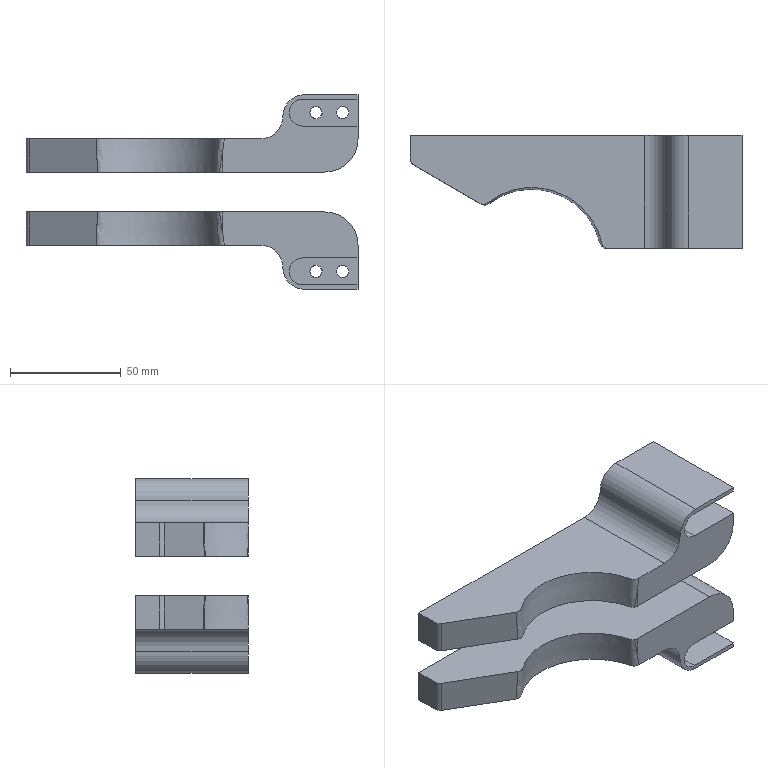NC program | NX | posted with a generic post | part box 150 x 51 x 88 mm
Lines 8834 to 9174 of 21241:
(ZLEVEL_PROFILE_COPY_COPY_COPY_1_COPY_COPY_COPY , TOOL : D12JING)
N17642 T11 M6
N17644 G54
N17646 G17 G0 G90 X62.688 Y-26.945 S9500 M3
N17648 G43 Z30. H11
N17650 Z-8.5
N17652 G94 G1 X61.043 Y-24.095 F1000.
N17654 G3 X60.005 Y-23.495 R1.199
N17656 G1 X-75. F1200.
N17658 G2 X-80.995 Y-17.5 R5.995
N17660 G1 Y-2.5
N17662 G2 X-75. Y3.495 R5.995
N17664 G1 X31.
N17666 G3 X35.005 Y7.5 R4.005
N17668 G2 X51. Y23.495 R15.995
N17670 G1 X75.
N17672 G2 X80.995 Y17.5 R5.995
N17674 G1 Y-2.5
N17676 G2 X60.005 Y-23.495 R20.995
N17678 G3 X58.966 Y-24.095 R1.199
N17680 G1 X57.237 Y-27.092
N17682 G0 X62.688 Y-26.945 Z-17.
N17684 G1 X61.043 Y-24.095 F1000.
N17686 G3 X60.005 Y-23.495 R1.199
N17688 G1 X-75. F1200.
N17690 G2 X-80.995 Y-17.5 R5.995
N17692 G1 Y-2.5
N17694 G2 X-75. Y3.495 R5.995
N17696 G1 X31.
N17698 G3 X35.005 Y7.5 R4.005
N17700 G2 X51. Y23.495 R15.995
N17702 G1 X75.
N17704 G2 X80.995 Y17.5 R5.995
N17706 G1 Y-2.5
N17708 G2 X60.005 Y-23.495 R20.995
N17710 G3 X58.966 Y-24.095 R1.199
N17712 G1 X57.237 Y-27.092
N17714 G0 X62.688 Y-26.945 Z-25.5
N17716 G1 X61.043 Y-24.095 F1000.
N17718 G3 X60.005 Y-23.495 R1.199
N17720 G1 X-75. F1200.
N17722 G2 X-80.995 Y-17.5 R5.995
N17724 G1 Y-2.5
N17726 G2 X-75. Y3.495 R5.995
N17728 G1 X31.
N17730 G3 X35.005 Y7.5 R4.005
N17732 G2 X51. Y23.495 R15.995
N17734 G1 X75.
N17736 G2 X80.995 Y17.5 R5.995
N17738 G1 Y-2.5
N17740 G2 X60.005 Y-23.495 R20.995
N17742 G3 X58.966 Y-24.095 R1.199
N17744 G1 X57.237 Y-27.092
N17746 G0 X62.688 Y-26.945 Z-34.
N17748 G1 X61.043 Y-24.095 F1000.
N17750 G3 X60.005 Y-23.495 R1.199
N17752 G1 X-75. F1200.
N17754 G2 X-80.995 Y-17.5 R5.995
N17756 G1 Y-2.5
N17758 G2 X-75. Y3.495 R5.995
N17760 G1 X31.
N17762 G3 X35.005 Y7.5 R4.005
N17764 G2 X51. Y23.495 R15.995
N17766 G1 X75.
N17768 G2 X80.995 Y17.5 R5.995
N17770 G1 Y-2.5
N17772 G2 X60.005 Y-23.495 R20.995
N17774 G3 X58.966 Y-24.095 R1.199
N17776 G1 X57.237 Y-27.092
N17778 G0 X62.688 Y-26.945 Z-42.5
N17780 G1 X61.043 Y-24.095 F1000.
N17782 G3 X60.005 Y-23.495 R1.199
N17784 G1 X-75. F1200.
N17786 G2 X-80.995 Y-17.5 R5.995
N17788 G1 Y-2.5
N17790 G2 X-75. Y3.495 R5.995
N17792 G1 X31.
N17794 G3 X35.005 Y7.5 R4.005
N17796 G2 X51. Y23.495 R15.995
N17798 G1 X75.
N17800 G2 X80.995 Y17.5 R5.995
N17802 G1 Y-2.5
N17804 G2 X60.005 Y-23.495 R20.995
N17806 G3 X58.966 Y-24.095 R1.199
N17808 G1 X57.237 Y-27.092
N17810 G0 X62.688 Y-26.945 Z-51.
N17812 G1 X61.043 Y-24.095 F1000.
N17814 G3 X60.005 Y-23.495 R1.199
N17816 G1 X-75. F1200.
N17818 G2 X-80.995 Y-17.5 R5.995
N17820 G1 Y-2.5
N17822 G2 X-75. Y3.495 R5.995
N17824 G1 X31.
N17826 G3 X35.005 Y7.5 R4.005
N17828 G2 X51. Y23.495 R15.995
N17830 G1 X75.
N17832 G2 X80.995 Y17.5 R5.995
N17834 G1 Y-2.5
N17836 G2 X60.005 Y-23.495 R20.995
N17838 G3 X58.966 Y-24.095 R1.199
N17840 G1 X57.237 Y-27.092
N17842 G0 Z30.
(ZLEVEL_PROFILE , TOOL : D12JING)
N17844 X81.455 Y9.508
N17846 Z0.
N17848 G1 Z-0.95 F1650.
N17850 X80.966 Y9.505
N17852 X74.609
N17854 X50.
N17856 G3 X49.895 Y9.4 R0.105
N17858 X50. Y9.295 R0.105
N17860 G1 X74.609
N17862 X80.966
N17864 X81.455 Y9.293
N17866 G3 X81.755 Y9.371 R0.6
N17868 G0 X81.455 Y9.508
N17870 G1 Z-1.9
N17872 X80.966 Y9.504
N17874 X74.609 Y9.505
N17876 X50.
N17878 G3 X49.895 Y9.4 R0.105
N17880 X50. Y9.295 R0.105
N17882 G1 X74.609
N17884 X80.966 Y9.296
N17886 X81.455 Y9.293
N17888 G3 X81.755 Y9.371 R0.6
N17890 G0 X81.455 Y9.508
N17892 G1 Z-2.85
N17894 X80.966 Y9.504
N17896 X74.609 Y9.505
N17898 X50.
N17900 G3 X49.895 Y9.4 R0.105
N17902 X50. Y9.295 R0.105
N17904 G1 X74.609
N17906 X80.966 Y9.296
N17908 X81.455 Y9.293
N17910 G3 X81.755 Y9.371 R0.6
N17912 G0 X81.455 Y9.508
N17914 G1 Z-3.8
N17916 X80.966 Y9.504
N17918 X75.098
N17920 X74.609 Y9.505
N17922 X50.
N17924 G3 X49.895 Y9.4 R0.105
N17926 X50. Y9.295 R0.105
N17928 G1 X74.609
N17930 X75.098 Y9.296
N17932 X80.966
N17934 X81.455 Y9.293
N17936 G3 X81.755 Y9.372 R0.6
N17938 G0 X81.455 Y9.508
N17940 G1 Z-4.75
N17942 X80.966 Y9.504
N17944 X75.098
N17946 X74.609 Y9.505
N17948 X50.
N17950 G3 X49.895 Y9.4 R0.105
N17952 X50. Y9.295 R0.105
N17954 G1 X74.609
N17956 X75.098 Y9.296
N17958 X80.966
N17960 X81.455 Y9.293
N17962 G3 X81.755 Y9.372 R0.6
N17964 G0 X81.455 Y9.508
N17966 G1 Z-5.7
N17968 X80.966 Y9.504
N17970 X75.098
N17972 X74.609 Y9.505
N17974 X50.
N17976 G3 X49.895 Y9.4 R0.105
N17978 X50. Y9.295 R0.105
N17980 G1 X74.609
N17982 X75.098 Y9.296
N17984 X80.966
N17986 X81.455 Y9.293
N17988 G3 X81.755 Y9.372 R0.6
N17990 G0 X81.455 Y9.507
N17992 G1 Z-6.65
N17994 X80.966 Y9.504
N17996 X75.098
N17998 X74.609 Y9.505
N18000 X50.
N18002 G3 X49.895 Y9.4 R0.105
N18004 X50. Y9.295 R0.105
N18006 G1 X74.609
N18008 X75.098 Y9.296
N18010 X80.966
N18012 X81.455 Y9.293
N18014 G3 X81.755 Y9.372 R0.6
N18016 G0 X81.455 Y9.507
N18018 G1 Z-7.6
N18020 X80.966 Y9.504
N18022 X75.098
N18024 X74.609 Y9.505
N18026 X50.
N18028 G3 X49.895 Y9.4 R0.105
N18030 X50. Y9.295 R0.105
N18032 G1 X74.609
N18034 X75.098 Y9.296
N18036 X80.966
N18038 X81.455 Y9.293
N18040 G3 X81.755 Y9.372 R0.6
N18042 G0 X81.455 Y9.507
N18044 G1 Z-8.55
N18046 X80.966 Y9.504
N18048 X75.098
N18050 X74.609 Y9.505
N18052 X50.
N18054 G3 X49.895 Y9.4 R0.105
N18056 X50. Y9.295 R0.105
N18058 G1 X74.609
N18060 X75.098 Y9.296
N18062 X80.966
N18064 X81.455 Y9.293
N18066 G3 X81.755 Y9.372 R0.6
N18068 G0 X81.455 Y9.507
N18070 G1 Z-9.5
N18072 X80.966 Y9.504
N18074 X75.098
N18076 X74.609 Y9.505
N18078 X50.
N18080 G3 X49.895 Y9.4 R0.105
N18082 X50. Y9.295 R0.105
N18084 G1 X74.609
N18086 X75.098 Y9.296
N18088 X80.966
N18090 X81.455 Y9.294
N18092 G3 X81.755 Y9.372 R0.6
N18094 G0 X81.455 Y9.507
N18096 G1 Z-10.45
N18098 X80.966 Y9.504
N18100 X75.098
N18102 X74.609 Y9.505
N18104 X50.
N18106 G3 X49.895 Y9.4 R0.105
N18108 X50. Y9.295 R0.105
N18110 G1 X74.609
N18112 X75.098 Y9.296
N18114 X80.966
N18116 X81.455 Y9.294
N18118 G3 X81.755 Y9.372 R0.6
N18120 G0 X81.455 Y9.507
N18122 G1 Z-11.4
N18124 X80.966 Y9.504
N18126 X75.098
N18128 X74.609 Y9.505
N18130 X50.
N18132 G3 X49.895 Y9.4 R0.105
N18134 X50. Y9.295 R0.105
N18136 G1 X74.609
N18138 X75.098 Y9.296
N18140 X80.966
N18142 X81.455 Y9.294
N18144 G3 X81.755 Y9.373 R0.6
N18146 G0 X81.455 Y9.507
N18148 G1 Z-12.35
N18150 X80.966 Y9.503
N18152 X75.098
N18154 X74.609 Y9.505
N18156 X50.
N18158 G3 X49.895 Y9.4 R0.105
N18160 X50. Y9.295 R0.105
N18162 G1 X74.609
N18164 X75.098 Y9.297
N18166 X80.966
N18168 X81.455 Y9.294
N18170 G3 X81.755 Y9.373 R0.6
N18172 G0 X81.455 Y9.507
N18174 G1 Z-13.3
N18176 X80.966 Y9.503
N18178 X75.098
N18180 X74.609 Y9.505
N18182 X50.
N18184 G3 X49.895 Y9.4 R0.105
N18186 X50. Y9.295 R0.105
N18188 G1 X74.609
N18190 X75.098 Y9.297
N18192 X80.966
N18194 X81.455 Y9.294
N18196 G3 X81.755 Y9.373 R0.6
N18198 G0 X81.455 Y9.507
N18200 G1 Z-14.25
N18202 X80.966 Y9.503
N18204 X75.098
N18206 X74.609 Y9.505
N18208 X50.
N18210 G3 X49.895 Y9.4 R0.105
N18212 X50. Y9.295 R0.105
N18214 G1 X74.609
N18216 X75.098 Y9.297
N18218 X80.966
N18220 X81.455 Y9.294
N18222 G3 X81.755 Y9.373 R0.6
N18224 G0 X81.455 Y9.507
N18226 G1 Z-15.2
N18228 X80.966 Y9.503
N18230 X75.098
N18232 X74.609 Y9.505
N18234 X50.
N18236 G3 X49.895 Y9.4 R0.105
N18238 X50. Y9.295 R0.105
N18240 G1 X74.609
N18242 X75.098 Y9.297
N18244 X80.966
N18246 X81.455 Y9.294
N18248 G3 X81.755 Y9.373 R0.6
N18250 G0 Z30.
N18252 M5
(PLANAR_MILL , TOOL : D6A45)
N18254 T07 M6
N18256 G54
N18258 G17 G0 G90 X15.635 Y-0.682 S9500 M3
N18260 G43 Z30. H7
N18262 Z0.
N18264 G94 G1 Z-1. F1250.
N18266 G3 X15.783 Y-1.6 R1.
N18268 G1 X31.
N18270 G3 X40.1 Y7.5 R9.1
N18272 G2 X51. Y18.4 R10.9
N18274 G1 X74.9
N18276 G2 X75.9 Y17.4 R1.
N18278 G1 Y15.6
N18280 G2 X74.9 Y14.6 R1.
N18282 G1 X50.
N18284 G3 X44.8 Y9.4 R5.2
N18286 X50. Y4.2 R5.2
N18288 G1 X74.9
N18290 G2 X75.9 Y3.2 R1.
N18292 G1 Y-2.5
N18294 G2 X60. Y-18.4 R15.9
N18296 G1 X14.976
N18298 G3 X14.827 Y-19.318 R1.
N18300 G1 Z0.
N18302 G0 Z30.
N18304 M5